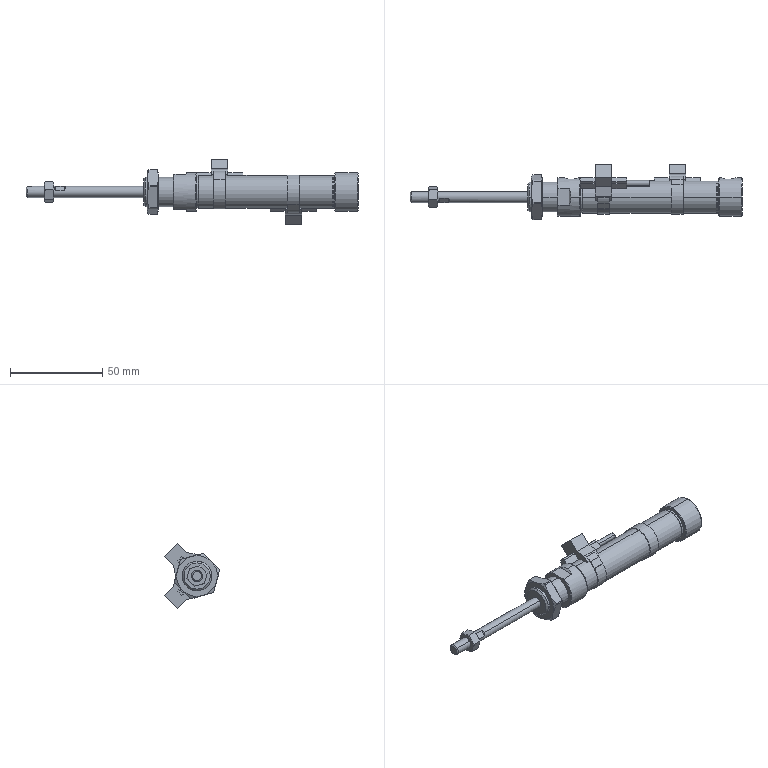Part | SolidWorks | 6 solids | 223 faces | box 179.68 x 29.769 x 35.214 mm | volume 28072 mm3 | plane 113 | cylinder 68 | cone 34 | torus 8 | commonest cylinder face diameters 17.4 x10 12.4 x8 18.4 x6 25 x6 1 x4 3 x4